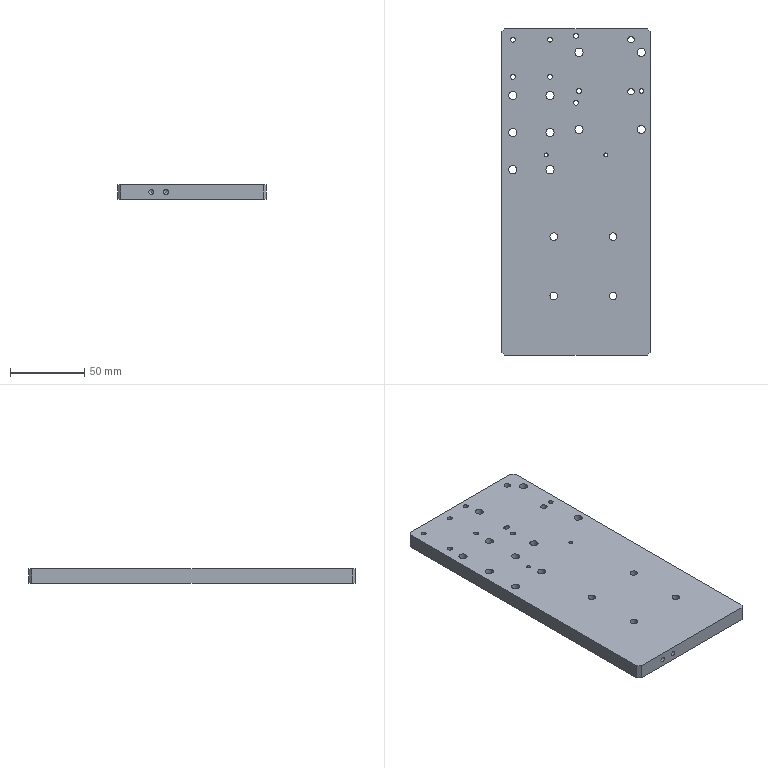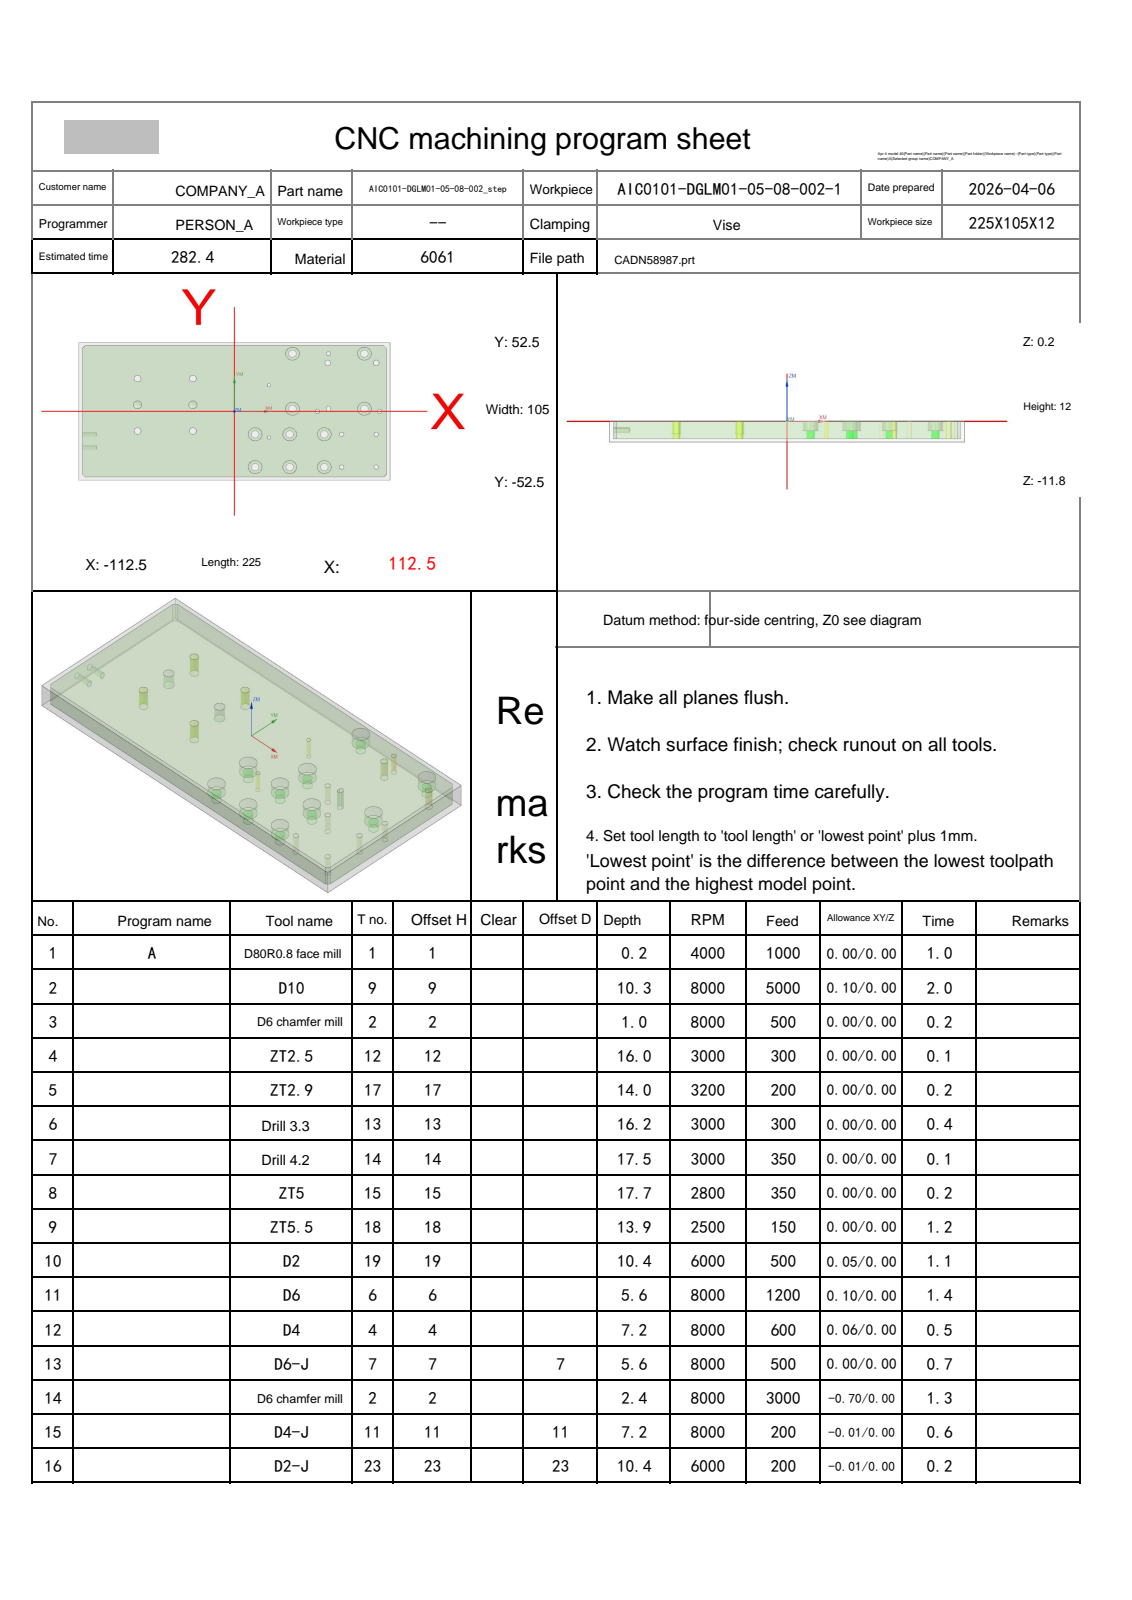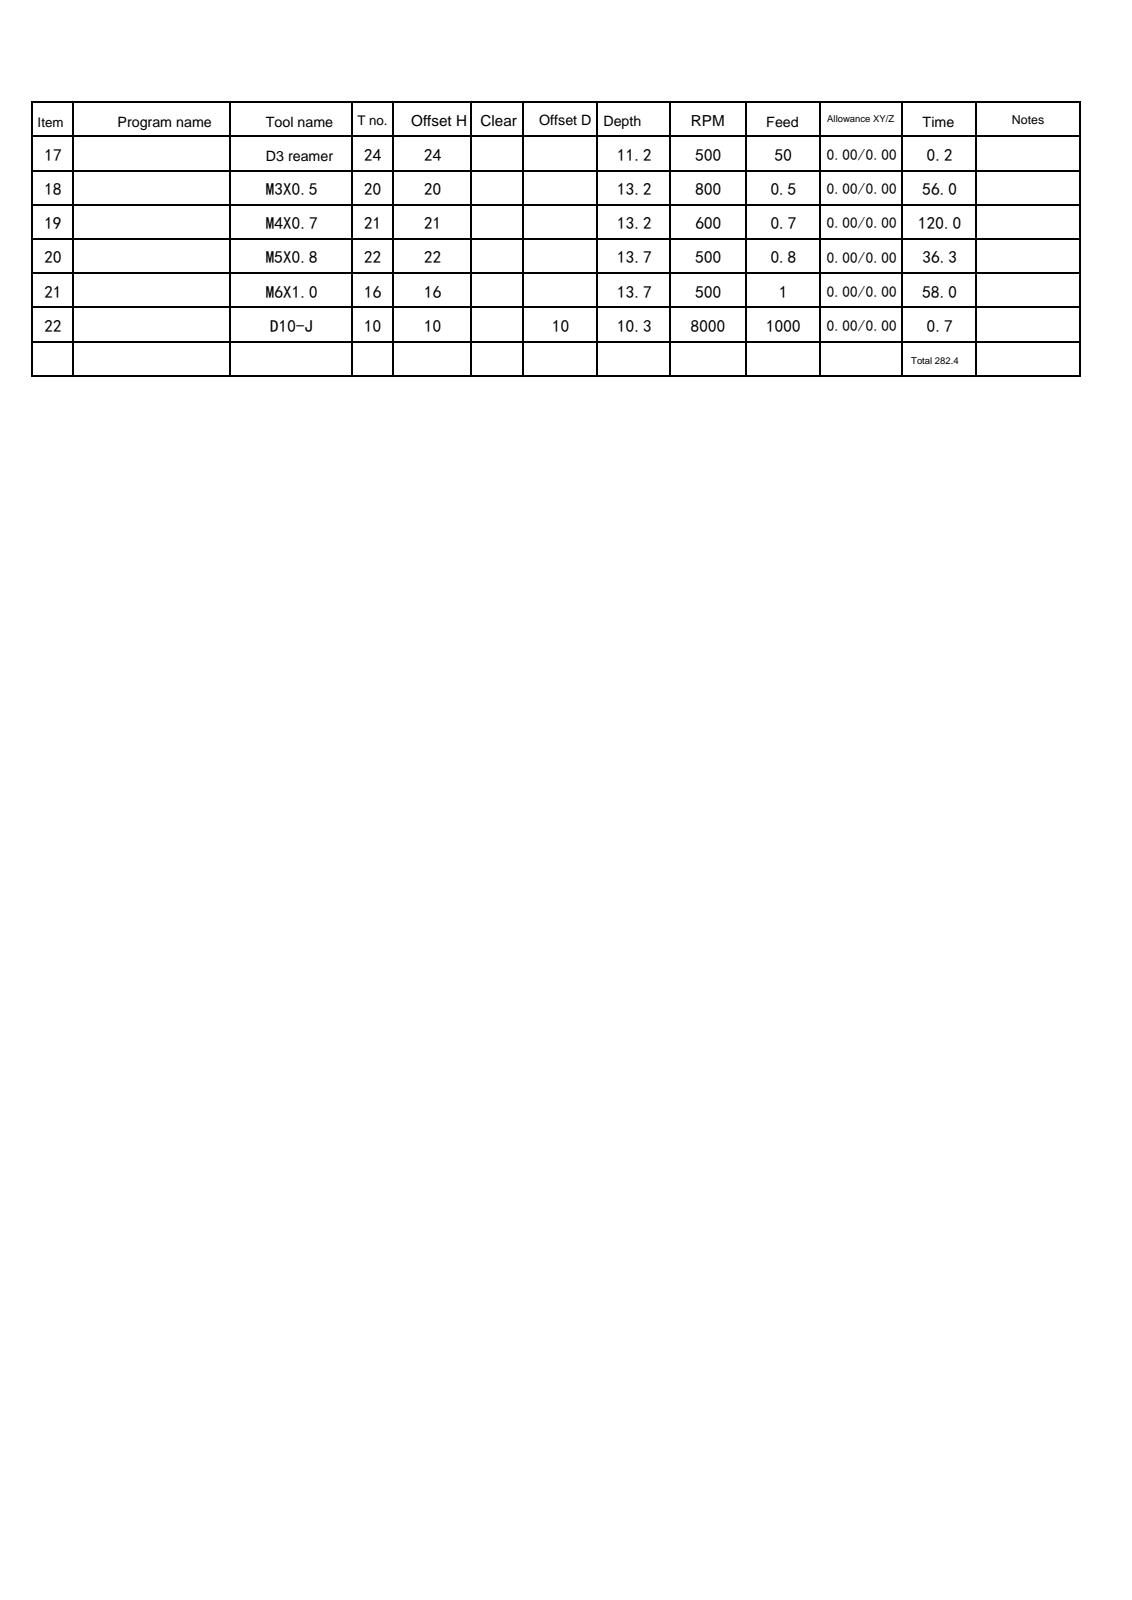NC program | NX | posted by the shop | part box 100 x 220 x 10 mm
Lines 1 to 1658 of 2500, first 1187 of 1656 lines:
%
O0001
(Machine time: 537.90 MIN)
(===Total Tool:21===)
(T1=D80R0.8 face mill D=80.  R=0.8  D-  H01 Z=-0.   )
(T9=D10     D=10.  R=0.   D-  H09 Z=-10.1 )
(T2=D6 chamfer mill   D=6.   R=0.   D-  H02 Z=-2.2  )
(T12=ZT2.5  D=2.5  DR_a=118 D-  H12 Z=-15.75)
(T17=ZT2.9  D=2.9  DR_a=120 D-  H17 Z=-13.84)
(T13=3.3 drill  D=3.3  DR_a=118 D-  H13 Z=-15.99)
(T14=4.2 drill  D=4.2  DR_a=118 D-  H14 Z=-17.26)
(T15=ZT5    D=5.   DR_a=118 D-  H15 Z=-17.5 )
(T18=ZT5.5  D=5.5  DR_a=118 D-  H18 Z=-13.65)
(T19=D2     D=2.   R=0.   D-  H19 Z=-10.2 )
(T6=D6      D=6.   R=0.   D-  H06 Z=-5.4  )
(T4=D4      D=4.   R=0.   D-  H04 Z=-7.   )
(T7=D6-J    D=6.   R=0.   D7  H07 Z=-5.4  )
(T11=D4-J   D=4.   R=0.   D11 H11 Z=-7.   )
(T23=D2-J   D=2.   R=0.   D23 H23 Z=-10.2 )
(T24=D3 reamer   D=3.   DR_a=180 D-  H24 Z=-11.  )
(T20=M3X0.5 D=2.5  DR_a=180 D-  H20 Z=-13.  )
(T21=M4X0.7 D=3.3  DR_a=180 D-  H21 Z=-13.  )
(T22=M5X0.8 D=4.2  DR_a=180 D-  H22 Z=-13.5 )
(T16=M6X1.0 D=5.   DR_a=180 D-  H16 Z=-13.5 )
(T10=D10-J  D=10.  R=0.   D10 H10 Z=-10.1 )
G80 G90 G17 G49 G40
G91 G28 Z0
M01
N1 T01 M06
(D80R0.8 face mill  D=80. R=0.8 H=01 ce=0.00 di=0.00)
G00 G90 G54 X-155. Y45. M03 S4000
G43 H01 Z20.
M08
Z2.
G01 Z0.0 F1000.
X-150.
X150.
Y0.0
X-150.
Y-45.
X150.
X155.
Z2.
G00 Z20.
G91 G28 Z0.0
M05
M09
G91 G28 Z0.0
M01
N2 T09 M06
(D10  D=10. R=0. H=09 ce=0.10 di=0.00)
G00 G90 G54 X0.0 Y55.1 M03 S8000
G43 H09 Z20.
M08
Z.5
G01 X108. Z.377 F5000.
G02 X111.606 Y53.606 Z.373 I0.0 J-5.1
G01 X113.606 Y51.606 Z.37
G02 X114.953 Y49.214 Z.367 I-3.606 J-3.606
X115.1 Y48. Z.365 I-4.953 J-1.214
G01 Y-48. Z.256
G02 X113.606 Y-51.606 Z.252 I-5.1 J0.0
G01 X111.606 Y-53.606 Z.249
G02 X108. Y-55.1 Z.244 I-3.606 J3.606
G01 X-108. Z-.001
G02 X-111.606 Y-53.606 Z-.006 I0.0 J5.1
G01 X-113.606 Y-51.606 Z-.009
G02 X-115.1 Y-48. Z-.013 I3.606 J3.606
G01 Y48. Z-.122
G02 X-113.606 Y51.606 Z-.127 I5.1 J0.0
G01 X-111.606 Y53.606 Z-.13
G02 X-108. Y55.1 Z-.135 I3.606 J-3.606
G01 X108. Z-.38
G02 X111.606 Y53.606 Z-.384 I0.0 J-5.1
G01 X113.606 Y51.606 Z-.387
G02 X114.953 Y49.214 Z-.391 I-3.606 J-3.606
X115.1 Y48. Z-.392 I-4.953 J-1.214
G01 Y-48. Z-.501
G02 X113.606 Y-51.606 Z-.505 I-5.1 J0.0
G01 X111.606 Y-53.606 Z-.509
G02 X108. Y-55.1 Z-.513 I-3.606 J3.606
G01 X-108. Z-.758
G02 X-111.606 Y-53.606 Z-.763 I0.0 J5.1
G01 X-113.606 Y-51.606 Z-.766
G02 X-115.1 Y-48. Z-.771 I3.606 J3.606
G01 Y48. Z-.879
G02 X-113.606 Y51.606 Z-.884 I5.1 J0.0
G01 X-111.606 Y53.606 Z-.887
G02 X-108. Y55.1 Z-.892 I3.606 J-3.606
G01 X108. Z-1.137
G02 X111.606 Y53.606 Z-1.141 I0.0 J-5.1
G01 X113.606 Y51.606 Z-1.145
G02 X114.953 Y49.214 Z-1.148 I-3.606 J-3.606
X115.1 Y48. Z-1.149 I-4.953 J-1.214
G01 Y-48. Z-1.258
G02 X113.606 Y-51.606 Z-1.263 I-5.1 J0.0
G01 X111.606 Y-53.606 Z-1.266
G02 X108. Y-55.1 Z-1.27 I-3.606 J3.606
G01 X-108. Z-1.515
G02 X-111.606 Y-53.606 Z-1.52 I0.0 J5.1
G01 X-113.606 Y-51.606 Z-1.523
G02 X-115.1 Y-48. Z-1.528 I3.606 J3.606
G01 Y48. Z-1.637
G02 X-113.606 Y51.606 Z-1.641 I5.1 J0.0
G01 X-111.606 Y53.606 Z-1.644
G02 X-108. Y55.1 Z-1.649 I3.606 J-3.606
G01 X108. Z-1.894
G02 X111.606 Y53.606 Z-1.899 I0.0 J-5.1
G01 X113.606 Y51.606 Z-1.902
G02 X114.953 Y49.214 Z-1.905 I-3.606 J-3.606
X115.1 Y48. Z-1.906 I-4.953 J-1.214
G01 Y-48. Z-2.015
G02 X113.606 Y-51.606 Z-2.02 I-5.1 J0.0
G01 X111.606 Y-53.606 Z-2.023
G02 X108. Y-55.1 Z-2.027 I-3.606 J3.606
G01 X-108. Z-2.273
G02 X-111.606 Y-53.606 Z-2.277 I0.0 J5.1
G01 X-113.606 Y-51.606 Z-2.28
G02 X-115.1 Y-48. Z-2.285 I3.606 J3.606
G01 Y48. Z-2.394
G02 X-113.606 Y51.606 Z-2.398 I5.1 J0.0
G01 X-111.606 Y53.606 Z-2.401
G02 X-108. Y55.1 Z-2.406 I3.606 J-3.606
G01 X108. Z-2.651
G02 X111.606 Y53.606 Z-2.656 I0.0 J-5.1
G01 X113.606 Y51.606 Z-2.659
G02 X114.953 Y49.214 Z-2.662 I-3.606 J-3.606
X115.1 Y48. Z-2.663 I-4.953 J-1.214
G01 Y-48. Z-2.772
G02 X113.606 Y-51.606 Z-2.777 I-5.1 J0.0
G01 X111.606 Y-53.606 Z-2.78
G02 X108. Y-55.1 Z-2.785 I-3.606 J3.606
G01 X-108. Z-3.03
G02 X-111.606 Y-53.606 Z-3.034 I0.0 J5.1
G01 X-113.606 Y-51.606 Z-3.037
G02 X-115.1 Y-48. Z-3.042 I3.606 J3.606
G01 Y48. Z-3.151
G02 X-113.606 Y51.606 Z-3.155 I5.1 J0.0
G01 X-111.606 Y53.606 Z-3.159
G02 X-108. Y55.1 Z-3.163 I3.606 J-3.606
G01 X108. Z-3.408
G02 X111.606 Y53.606 Z-3.413 I0.0 J-5.1
G01 X113.606 Y51.606 Z-3.416
G02 X114.953 Y49.214 Z-3.419 I-3.606 J-3.606
X115.1 Y48. Z-3.421 I-4.953 J-1.214
G01 Y-48. Z-3.529
G02 X113.606 Y-51.606 Z-3.534 I-5.1 J0.0
G01 X111.606 Y-53.606 Z-3.537
G02 X108. Y-55.1 Z-3.542 I-3.606 J3.606
G01 X-108. Z-3.787
G02 X-111.606 Y-53.606 Z-3.791 I0.0 J5.1
G01 X-113.606 Y-51.606 Z-3.795
G02 X-115.1 Y-48. Z-3.799 I3.606 J3.606
G01 Y48. Z-3.908
G02 X-113.606 Y51.606 Z-3.913 I5.1 J0.0
G01 X-111.606 Y53.606 Z-3.916
G02 X-108. Y55.1 Z-3.92 I3.606 J-3.606
G01 X108. Z-4.165
G02 X111.606 Y53.606 Z-4.17 I0.0 J-5.1
G01 X113.606 Y51.606 Z-4.173
G02 X114.953 Y49.214 Z-4.176 I-3.606 J-3.606
X115.1 Y48. Z-4.178 I-4.953 J-1.214
G01 Y-48. Z-4.287
G02 X113.606 Y-51.606 Z-4.291 I-5.1 J0.0
G01 X111.606 Y-53.606 Z-4.294
G02 X108. Y-55.1 Z-4.299 I-3.606 J3.606
G01 X-108. Z-4.544
G02 X-111.606 Y-53.606 Z-4.549 I0.0 J5.1
G01 X-113.606 Y-51.606 Z-4.552
G02 X-115.1 Y-48. Z-4.556 I3.606 J3.606
G01 Y48. Z-4.665
G02 X-113.606 Y51.606 Z-4.67 I5.1 J0.0
G01 X-111.606 Y53.606 Z-4.673
G02 X-108. Y55.1 Z-4.677 I3.606 J-3.606
G01 X108. Z-4.923
G02 X111.606 Y53.606 Z-4.927 I0.0 J-5.1
G01 X113.606 Y51.606 Z-4.93
G02 X114.953 Y49.214 Z-4.933 I-3.606 J-3.606
X115.1 Y48. Z-4.935 I-4.953 J-1.214
G01 Y-48. Z-5.044
G02 X113.606 Y-51.606 Z-5.048 I-5.1 J0.0
G01 X111.606 Y-53.606 Z-5.051
G02 X108. Y-55.1 Z-5.056 I-3.606 J3.606
G01 X-108. Z-5.301
G02 X-111.606 Y-53.606 Z-5.306 I0.0 J5.1
G01 X-113.606 Y-51.606 Z-5.309
G02 X-115.1 Y-48. Z-5.313 I3.606 J3.606
G01 Y48. Z-5.422
G02 X-113.606 Y51.606 Z-5.427 I5.1 J0.0
G01 X-111.606 Y53.606 Z-5.43
G02 X-108. Y55.1 Z-5.435 I3.606 J-3.606
G01 X108. Z-5.68
G02 X111.606 Y53.606 Z-5.684 I0.0 J-5.1
G01 X113.606 Y51.606 Z-5.687
G02 X114.953 Y49.214 Z-5.691 I-3.606 J-3.606
X115.1 Y48. Z-5.692 I-4.953 J-1.214
G01 Y-48. Z-5.801
G02 X113.606 Y-51.606 Z-5.805 I-5.1 J0.0
G01 X111.606 Y-53.606 Z-5.809
G02 X108. Y-55.1 Z-5.813 I-3.606 J3.606
G01 X-108. Z-6.058
G02 X-111.606 Y-53.606 Z-6.063 I0.0 J5.1
G01 X-113.606 Y-51.606 Z-6.066
G02 X-115.1 Y-48. Z-6.071 I3.606 J3.606
G01 Y48. Z-6.179
G02 X-113.606 Y51.606 Z-6.184 I5.1 J0.0
G01 X-111.606 Y53.606 Z-6.187
G02 X-108. Y55.1 Z-6.192 I3.606 J-3.606
G01 X108. Z-6.437
G02 X111.606 Y53.606 Z-6.441 I0.0 J-5.1
G01 X113.606 Y51.606 Z-6.445
G02 X114.953 Y49.214 Z-6.448 I-3.606 J-3.606
X115.1 Y48. Z-6.449 I-4.953 J-1.214
G01 Y-48. Z-6.558
G02 X113.606 Y-51.606 Z-6.563 I-5.1 J0.0
G01 X111.606 Y-53.606 Z-6.566
G02 X108. Y-55.1 Z-6.57 I-3.606 J3.606
G01 X-108. Z-6.815
G02 X-111.606 Y-53.606 Z-6.82 I0.0 J5.1
G01 X-113.606 Y-51.606 Z-6.823
G02 X-115.1 Y-48. Z-6.828 I3.606 J3.606
G01 Y48. Z-6.937
G02 X-113.606 Y51.606 Z-6.941 I5.1 J0.0
G01 X-111.606 Y53.606 Z-6.944
G02 X-108. Y55.1 Z-6.949 I3.606 J-3.606
G01 X108. Z-7.194
G02 X111.606 Y53.606 Z-7.199 I0.0 J-5.1
G01 X113.606 Y51.606 Z-7.202
G02 X114.953 Y49.214 Z-7.205 I-3.606 J-3.606
X115.1 Y48. Z-7.206 I-4.953 J-1.214
G01 Y-48. Z-7.315
G02 X113.606 Y-51.606 Z-7.32 I-5.1 J0.0
G01 X111.606 Y-53.606 Z-7.323
G02 X108. Y-55.1 Z-7.327 I-3.606 J3.606
G01 X-108. Z-7.573
G02 X-111.606 Y-53.606 Z-7.577 I0.0 J5.1
G01 X-113.606 Y-51.606 Z-7.58
G02 X-115.1 Y-48. Z-7.585 I3.606 J3.606
G01 Y48. Z-7.694
G02 X-113.606 Y51.606 Z-7.698 I5.1 J0.0
G01 X-111.606 Y53.606 Z-7.701
G02 X-108. Y55.1 Z-7.706 I3.606 J-3.606
G01 X108. Z-7.951
G02 X111.606 Y53.606 Z-7.956 I0.0 J-5.1
G01 X113.606 Y51.606 Z-7.959
G02 X114.953 Y49.214 Z-7.962 I-3.606 J-3.606
X115.1 Y48. Z-7.963 I-4.953 J-1.214
G01 Y-48. Z-8.072
G02 X113.606 Y-51.606 Z-8.077 I-5.1 J0.0
G01 X111.606 Y-53.606 Z-8.08
G02 X108. Y-55.1 Z-8.085 I-3.606 J3.606
G01 X-108. Z-8.33
G02 X-111.606 Y-53.606 Z-8.334 I0.0 J5.1
G01 X-113.606 Y-51.606 Z-8.337
G02 X-115.1 Y-48. Z-8.342 I3.606 J3.606
G01 Y48. Z-8.451
G02 X-113.606 Y51.606 Z-8.455 I5.1 J0.0
G01 X-111.606 Y53.606 Z-8.459
G02 X-108. Y55.1 Z-8.463 I3.606 J-3.606
G01 X108. Z-8.708
G02 X111.606 Y53.606 Z-8.713 I0.0 J-5.1
G01 X113.606 Y51.606 Z-8.716
G02 X114.953 Y49.214 Z-8.719 I-3.606 J-3.606
X115.1 Y48. Z-8.721 I-4.953 J-1.214
G01 Y-48. Z-8.829
G02 X113.606 Y-51.606 Z-8.834 I-5.1 J0.0
G01 X111.606 Y-53.606 Z-8.837
G02 X108. Y-55.1 Z-8.842 I-3.606 J3.606
G01 X-108. Z-9.087
G02 X-111.606 Y-53.606 Z-9.091 I0.0 J5.1
G01 X-113.606 Y-51.606 Z-9.095
G02 X-115.1 Y-48. Z-9.099 I3.606 J3.606
G01 Y48. Z-9.208
G02 X-113.606 Y51.606 Z-9.213 I5.1 J0.0
G01 X-111.606 Y53.606 Z-9.216
G02 X-108. Y55.1 Z-9.22 I3.606 J-3.606
G01 X108. Z-9.465
G02 X111.606 Y53.606 Z-9.47 I0.0 J-5.1
G01 X113.606 Y51.606 Z-9.473
G02 X114.953 Y49.214 Z-9.476 I-3.606 J-3.606
X115.1 Y48. Z-9.478 I-4.953 J-1.214
G01 Y-48. Z-9.587
G02 X113.606 Y-51.606 Z-9.591 I-5.1 J0.0
G01 X111.606 Y-53.606 Z-9.594
G02 X108. Y-55.1 Z-9.599 I-3.606 J3.606
G01 X-108. Z-9.844
G02 X-111.606 Y-53.606 Z-9.849 I0.0 J5.1
G01 X-113.606 Y-51.606 Z-9.852
G02 X-115.1 Y-48. Z-9.856 I3.606 J3.606
G01 Y48. Z-9.965
G02 X-113.606 Y51.606 Z-9.97 I5.1 J0.0
G01 X-111.606 Y53.606 Z-9.973
G02 X-108. Y55.1 Z-9.977 I3.606 J-3.606
G01 X0.0 Z-10.1
X108.
G02 X111.606 Y53.606 I0.0 J-5.1
G01 X113.606 Y51.606
G02 X115.1 Y48. I-3.606 J-3.606
G01 Y-48.
G02 X113.606 Y-51.606 I-5.1 J0.0
G01 X111.606 Y-53.606
G02 X108. Y-55.1 I-3.606 J3.606
G01 X-108.
G02 X-111.606 Y-53.606 I0.0 J5.1
G01 X-113.606 Y-51.606
G02 X-115.1 Y-48. I3.606 J3.606
G01 Y48.
G02 X-113.606 Y51.606 I5.1 J0.0
G01 X-111.606 Y53.606
G02 X-108. Y55.1 I3.606 J-3.606
G01 X0.0
X.5
Z-9.1
G00 Z20.
G91 G28 Z0.0
M05
M09
G91 G28 Z0.0
M01
N3 T02 M06
(D6 chamfer mill  D=6. R=0. H=02 ce=0.00 di=0.00)
G00 G90 G54 X102.5 Y37. M03 S8000
G43 H02 Z20.
M08
G98 G81 X102.5 Y37. Z-.8 R1. F500.
X94. Y44.
X68.
X67.5 Y37.
X42. Y44.
X25. Y20.
X42. Y2.
X60. Y0.0
X65. Y-17.5
X77.5
X94. Y2.
X105. Y0.0
X102.5 Y-17.5
Y-42.5
X77.5
X65.
X40.
Y-17.5
X25. Y-20.
X15. Y-17.5
Y-42.5
X-30. Y-15.
Y5.
Y25.
X-70.
Y5.
Y-15.
X68. Y2.5
G80
G00 Z20.
G91 G28 Z0.0
M05
M09
G91 G28 Z0.0
M01
N4 T12 M06
(ZT2.5 D=2.5 DR_a=118 H=12)
G00 G90 G54 X25. Y-20. M03 S3000
G43 H12 Z20.
M08
G98 G83 X25. Y-20. Z-15.751 R1. F300. Q2.
Y20.
G80
G00 Z20.
G91 G28 Z0.0
M05
M09
G91 G28 Z0.0
M01
N5 T17 M06
(ZT2.9 D=2.9 DR_a=120 H=17)
G00 G90 G54 X68. Y44. M03 S3200
G43 H17 Z20.
M08
G98 G83 X68. Y44. Z-13.837 R1. F200. Q2.
Y2.5
G80
G00 Z20.
G91 G28 Z0.0
M05
M09
G91 G28 Z0.0
M01
N6 T13 M06
(3.3 drill D=3.3 DR_a=118 H=13)
G00 G90 G54 X60. Y0.0 M03 S3000
G43 H13 Z20.
M08
G98 G83 X60. Y0.0 Z-15.991 R1. F300. Q2.
X77.5 Y-17.5
Y-42.5
X102.5
Y-17.5
X105. Y0.0
G80
G00 Z20.
G91 G28 Z0.0
M05
M09
G91 G28 Z0.0
M01
N7 T14 M06
(4.2 drill D=4.2 DR_a=118 H=14)
G00 G90 G54 X67.5 Y37. M03 S3000
G43 H14 Z20.
M08
G98 G83 X67.5 Y37. Z-17.262 R1. F350. Q3.
X102.5
G80
G00 Z20.
G91 G28 Z0.0
M05
M09
G91 G28 Z0.0
M01
N8 T15 M06
(ZT5 D=5. DR_a=118 H=15)
G00 G90 G54 X-30. Y25. M03 S2800
G43 H15 Z20.
M08
G98 G83 X-30. Y25. Z-17.502 R1. F350. Q3.
X-70.
Y-15.
X-30.
G80
G00 Z20.
G91 G28 Z0.0
M05
M09
G91 G28 Z0.0
M01
N9 T18 M06
(ZT5.5 D=5.5 DR_a=118 H=18)
G00 G90 G54 X42. Y44. M03 S1200
G43 H18 Z20.
M08
G98 G83 X42. Y44. Z-13.652 R1. F150. Q2.
Y2.
X40. Y-17.5
X15.
Y-42.5
X40.
X65.
Y-17.5
X94. Y2.
Y44.
G80
G00 Z20.
G00 G90 X-30. Y5. M03 S2500
Z20.
G98 G83 X-30. Y5. Z-8.703 R1. F150. Q2.
X-70.
G80
G00 Z20.
G91 G28 Z0.0
M05
M09
G91 G28 Z0.0
M01
N10 T19 M06
(D2  D=2. R=0. H=19 ce=0.05 di=0.00)
G00 G90 G54 X68.45 Y2. M03 S6000
G43 H19 Z20.
M08
Z.5
G01 Y2.5 Z.49 F500.
G03 X68. Y2.95 Z.475 I-.45 J0.0
X67.55 Y2.5 Z.46 I0.0 J-.45
G01 Y1.5 Z.44
G03 X68. Y1.05 Z.425 I.45 J0.0
X68.45 Y1.5 Z.41 I0.0 J.45
G01 Y2.5 Z.39
G03 X68. Y2.95 Z.375 I-.45 J0.0
X67.55 Y2.5 Z.36 I0.0 J-.45
G01 Y1.5 Z.34
G03 X68. Y1.05 Z.325 I.45 J0.0
X68.45 Y1.5 Z.31 I0.0 J.45
G01 Y2.5 Z.29
G03 X68. Y2.95 Z.275 I-.45 J0.0
X67.55 Y2.5 Z.26 I0.0 J-.45
G01 Y1.5 Z.24
G03 X68. Y1.05 Z.225 I.45 J0.0
X68.45 Y1.5 Z.21 I0.0 J.45
G01 Y2.5 Z.19
G03 X68. Y2.95 Z.175 I-.45 J0.0
X67.55 Y2.5 Z.16 I0.0 J-.45
G01 Y1.5 Z.14
G03 X68. Y1.05 Z.125 I.45 J0.0
X68.45 Y1.5 Z.11 I0.0 J.45
G01 Y2.5 Z.09
G03 X68. Y2.95 Z.075 I-.45 J0.0
X67.55 Y2.5 Z.06 I0.0 J-.45
G01 Y1.5 Z.04
G03 X68. Y1.05 Z.025 I.45 J0.0
X68.45 Y1.5 Z.01 I0.0 J.45
G01 Y2.5 Z-.01
G03 X68. Y2.95 Z-.025 I-.45 J0.0
X67.55 Y2.5 Z-.04 I0.0 J-.45
G01 Y1.5 Z-.06
G03 X68. Y1.05 Z-.075 I.45 J0.0
X68.45 Y1.5 Z-.09 I0.0 J.45
G01 Y2.5 Z-.11
G03 X68. Y2.95 Z-.125 I-.45 J0.0
X67.55 Y2.5 Z-.14 I0.0 J-.45
G01 Y1.5 Z-.16
G03 X68. Y1.05 Z-.175 I.45 J0.0
X68.45 Y1.5 Z-.19 I0.0 J.45
G01 Y2.5 Z-.21
G03 X68. Y2.95 Z-.225 I-.45 J0.0
X67.55 Y2.5 Z-.24 I0.0 J-.45
G01 Y1.5 Z-.26
G03 X68. Y1.05 Z-.275 I.45 J0.0
X68.45 Y1.5 Z-.29 I0.0 J.45
G01 Y2.5 Z-.31
G03 X68. Y2.95 Z-.325 I-.45 J0.0
X67.55 Y2.5 Z-.34 I0.0 J-.45
G01 Y1.5 Z-.36
G03 X68. Y1.05 Z-.375 I.45 J0.0
X68.45 Y1.5 Z-.39 I0.0 J.45
G01 Y2.5 Z-.41
G03 X68. Y2.95 Z-.425 I-.45 J0.0
X67.55 Y2.5 Z-.44 I0.0 J-.45
G01 Y1.5 Z-.46
G03 X68. Y1.05 Z-.475 I.45 J0.0
X68.45 Y1.5 Z-.49 I0.0 J.45
G01 Y2.5 Z-.51
G03 X68. Y2.95 Z-.525 I-.45 J0.0
X67.55 Y2.5 Z-.54 I0.0 J-.45
G01 Y1.5 Z-.56
G03 X68. Y1.05 Z-.575 I.45 J0.0
X68.45 Y1.5 Z-.59 I0.0 J.45
G01 Y2.5 Z-.61
G03 X68. Y2.95 Z-.625 I-.45 J0.0
X67.55 Y2.5 Z-.64 I0.0 J-.45
G01 Y1.5 Z-.66
G03 X68. Y1.05 Z-.675 I.45 J0.0
X68.45 Y1.5 Z-.69 I0.0 J.45
G01 Y2.5 Z-.71
G03 X68. Y2.95 Z-.725 I-.45 J0.0
X67.55 Y2.5 Z-.74 I0.0 J-.45
G01 Y1.5 Z-.76
G03 X68. Y1.05 Z-.775 I.45 J0.0
X68.45 Y1.5 Z-.79 I0.0 J.45
G01 Y2.5 Z-.81
G03 X68. Y2.95 Z-.825 I-.45 J0.0
X67.55 Y2.5 Z-.84 I0.0 J-.45
G01 Y1.5 Z-.86
G03 X68. Y1.05 Z-.875 I.45 J0.0
X68.45 Y1.5 Z-.89 I0.0 J.45
G01 Y2.5 Z-.91
G03 X68. Y2.95 Z-.925 I-.45 J0.0
X67.55 Y2.5 Z-.94 I0.0 J-.45
G01 Y1.5 Z-.96
G03 X68. Y1.05 Z-.975 I.45 J0.0
X68.45 Y1.5 Z-.99 I0.0 J.45
G01 Y2.5 Z-1.01
G03 X68. Y2.95 Z-1.025 I-.45 J0.0
X67.55 Y2.5 Z-1.04 I0.0 J-.45
G01 Y1.5 Z-1.06
G03 X68. Y1.05 Z-1.075 I.45 J0.0
X68.45 Y1.5 Z-1.09 I0.0 J.45
G01 Y2.5 Z-1.11
G03 X68. Y2.95 Z-1.125 I-.45 J0.0
X67.55 Y2.5 Z-1.14 I0.0 J-.45
G01 Y1.5 Z-1.16
G03 X68. Y1.05 Z-1.175 I.45 J0.0
X68.45 Y1.5 Z-1.19 I0.0 J.45
G01 Y2.5 Z-1.21
G03 X68. Y2.95 Z-1.225 I-.45 J0.0
X67.55 Y2.5 Z-1.24 I0.0 J-.45
G01 Y1.5 Z-1.26
G03 X68. Y1.05 Z-1.275 I.45 J0.0
X68.45 Y1.5 Z-1.29 I0.0 J.45
G01 Y2.5 Z-1.31
G03 X68. Y2.95 Z-1.325 I-.45 J0.0
X67.55 Y2.5 Z-1.34 I0.0 J-.45
G01 Y1.5 Z-1.36
G03 X68. Y1.05 Z-1.375 I.45 J0.0
X68.45 Y1.5 Z-1.39 I0.0 J.45
G01 Y2.5 Z-1.41
G03 X68. Y2.95 Z-1.425 I-.45 J0.0
X67.55 Y2.5 Z-1.44 I0.0 J-.45
G01 Y1.5 Z-1.46
G03 X68. Y1.05 Z-1.475 I.45 J0.0
X68.45 Y1.5 Z-1.49 I0.0 J.45
G01 Y2.5 Z-1.51
G03 X68. Y2.95 Z-1.525 I-.45 J0.0
X67.55 Y2.5 Z-1.54 I0.0 J-.45
G01 Y1.5 Z-1.56
G03 X68. Y1.05 Z-1.575 I.45 J0.0
X68.45 Y1.5 Z-1.59 I0.0 J.45
G01 Y2.5 Z-1.61
G03 X68. Y2.95 Z-1.625 I-.45 J0.0
X67.55 Y2.5 Z-1.64 I0.0 J-.45
G01 Y1.5 Z-1.66
G03 X68. Y1.05 Z-1.675 I.45 J0.0
X68.45 Y1.5 Z-1.69 I0.0 J.45
G01 Y2.5 Z-1.71
G03 X68. Y2.95 Z-1.725 I-.45 J0.0
X67.55 Y2.5 Z-1.74 I0.0 J-.45
G01 Y1.5 Z-1.76
G03 X68. Y1.05 Z-1.775 I.45 J0.0
X68.45 Y1.5 Z-1.79 I0.0 J.45
G01 Y2.5 Z-1.81
G03 X68. Y2.95 Z-1.825 I-.45 J0.0
X67.55 Y2.5 Z-1.84 I0.0 J-.45
G01 Y1.5 Z-1.86
G03 X68. Y1.05 Z-1.875 I.45 J0.0
X68.45 Y1.5 Z-1.89 I0.0 J.45
G01 Y2.5 Z-1.91
G03 X68. Y2.95 Z-1.925 I-.45 J0.0
X67.55 Y2.5 Z-1.94 I0.0 J-.45
G01 Y1.5 Z-1.96
G03 X68. Y1.05 Z-1.975 I.45 J0.0
X68.45 Y1.5 Z-1.99 I0.0 J.45
G01 Y2.5 Z-2.01
G03 X68. Y2.95 Z-2.025 I-.45 J0.0
X67.55 Y2.5 Z-2.04 I0.0 J-.45
G01 Y1.5 Z-2.06
G03 X68. Y1.05 Z-2.075 I.45 J0.0
X68.45 Y1.5 Z-2.09 I0.0 J.45
G01 Y2.5 Z-2.11
G03 X68. Y2.95 Z-2.125 I-.45 J0.0
X67.55 Y2.5 Z-2.14 I0.0 J-.45
G01 Y1.5 Z-2.16
G03 X68. Y1.05 Z-2.175 I.45 J0.0
X68.45 Y1.5 Z-2.19 I0.0 J.45
G01 Y2.5 Z-2.21
G03 X68. Y2.95 Z-2.225 I-.45 J0.0
X67.55 Y2.5 Z-2.24 I0.0 J-.45
G01 Y1.5 Z-2.26
G03 X68. Y1.05 Z-2.275 I.45 J0.0
X68.45 Y1.5 Z-2.29 I0.0 J.45
G01 Y2.5 Z-2.31
G03 X68. Y2.95 Z-2.325 I-.45 J0.0
X67.55 Y2.5 Z-2.34 I0.0 J-.45
G01 Y1.5 Z-2.36
G03 X68. Y1.05 Z-2.375 I.45 J0.0
X68.45 Y1.5 Z-2.39 I0.0 J.45
G01 Y2.5 Z-2.41
G03 X68. Y2.95 Z-2.425 I-.45 J0.0
X67.55 Y2.5 Z-2.44 I0.0 J-.45
G01 Y1.5 Z-2.46
G03 X68. Y1.05 Z-2.475 I.45 J0.0
X68.45 Y1.5 Z-2.49 I0.0 J.45
G01 Y2.5 Z-2.51
G03 X68. Y2.95 Z-2.525 I-.45 J0.0
X67.55 Y2.5 Z-2.54 I0.0 J-.45
G01 Y1.5 Z-2.56
G03 X68. Y1.05 Z-2.575 I.45 J0.0
X68.45 Y1.5 Z-2.59 I0.0 J.45
G01 Y2.5 Z-2.61
G03 X68. Y2.95 Z-2.625 I-.45 J0.0
X67.55 Y2.5 Z-2.64 I0.0 J-.45
G01 Y1.5 Z-2.66
G03 X68. Y1.05 Z-2.675 I.45 J0.0
X68.45 Y1.5 Z-2.69 I0.0 J.45
G01 Y2.5 Z-2.71
G03 X68. Y2.95 Z-2.725 I-.45 J0.0
X67.55 Y2.5 Z-2.74 I0.0 J-.45
G01 Y1.5 Z-2.76
G03 X68. Y1.05 Z-2.775 I.45 J0.0
X68.45 Y1.5 Z-2.79 I0.0 J.45
G01 Y2.5 Z-2.81
G03 X68. Y2.95 Z-2.825 I-.45 J0.0
X67.55 Y2.5 Z-2.84 I0.0 J-.45
G01 Y1.5 Z-2.86
G03 X68. Y1.05 Z-2.875 I.45 J0.0
X68.45 Y1.5 Z-2.89 I0.0 J.45
G01 Y2.5 Z-2.91
G03 X68. Y2.95 Z-2.925 I-.45 J0.0
X67.55 Y2.5 Z-2.94 I0.0 J-.45
G01 Y1.5 Z-2.96
G03 X68. Y1.05 Z-2.975 I.45 J0.0
X68.45 Y1.5 Z-2.99 I0.0 J.45
G01 Y2.5 Z-3.01
G03 X68. Y2.95 Z-3.025 I-.45 J0.0
X67.55 Y2.5 Z-3.04 I0.0 J-.45
G01 Y1.5 Z-3.06
G03 X68. Y1.05 Z-3.075 I.45 J0.0
X68.45 Y1.5 Z-3.09 I0.0 J.45
G01 Y2.5 Z-3.11
G03 X68. Y2.95 Z-3.125 I-.45 J0.0
X67.55 Y2.5 Z-3.14 I0.0 J-.45
G01 Y1.5 Z-3.16
G03 X68. Y1.05 Z-3.175 I.45 J0.0
X68.45 Y1.5 Z-3.19 I0.0 J.45
G01 Y2.5 Z-3.21
G03 X68. Y2.95 Z-3.225 I-.45 J0.0
X67.55 Y2.5 Z-3.24 I0.0 J-.45
G01 Y1.5 Z-3.26
G03 X68. Y1.05 Z-3.275 I.45 J0.0
X68.45 Y1.5 Z-3.29 I0.0 J.45
G01 Y2.5 Z-3.31
G03 X68. Y2.95 Z-3.325 I-.45 J0.0
X67.55 Y2.5 Z-3.34 I0.0 J-.45
G01 Y1.5 Z-3.36
G03 X68. Y1.05 Z-3.375 I.45 J0.0
X68.45 Y1.5 Z-3.39 I0.0 J.45
G01 Y2.5 Z-3.41
G03 X68. Y2.95 Z-3.425 I-.45 J0.0
X67.55 Y2.5 Z-3.44 I0.0 J-.45
G01 Y1.5 Z-3.46
G03 X68. Y1.05 Z-3.475 I.45 J0.0
X68.45 Y1.5 Z-3.49 I0.0 J.45
G01 Y2.5 Z-3.51
G03 X68. Y2.95 Z-3.525 I-.45 J0.0
X67.55 Y2.5 Z-3.54 I0.0 J-.45
G01 Y1.5 Z-3.56
G03 X68. Y1.05 Z-3.575 I.45 J0.0
X68.45 Y1.5 Z-3.59 I0.0 J.45
G01 Y2.5 Z-3.61
G03 X68. Y2.95 Z-3.625 I-.45 J0.0
X67.55 Y2.5 Z-3.64 I0.0 J-.45
G01 Y1.5 Z-3.66
G03 X68. Y1.05 Z-3.675 I.45 J0.0
X68.45 Y1.5 Z-3.69 I0.0 J.45
G01 Y2.5 Z-3.71
G03 X68. Y2.95 Z-3.725 I-.45 J0.0
X67.55 Y2.5 Z-3.74 I0.0 J-.45
G01 Y1.5 Z-3.76
G03 X68. Y1.05 Z-3.775 I.45 J0.0
X68.45 Y1.5 Z-3.79 I0.0 J.45
G01 Y2.5 Z-3.81
G03 X68. Y2.95 Z-3.825 I-.45 J0.0
X67.55 Y2.5 Z-3.84 I0.0 J-.45
G01 Y1.5 Z-3.86
G03 X68. Y1.05 Z-3.875 I.45 J0.0
X68.45 Y1.5 Z-3.89 I0.0 J.45
G01 Y2.5 Z-3.91
G03 X68. Y2.95 Z-3.925 I-.45 J0.0
X67.55 Y2.5 Z-3.94 I0.0 J-.45
G01 Y1.5 Z-3.96
G03 X68. Y1.05 Z-3.975 I.45 J0.0
X68.45 Y1.5 Z-3.99 I0.0 J.45
G01 Y2.5 Z-4.01
G03 X68. Y2.95 Z-4.025 I-.45 J0.0
X67.55 Y2.5 Z-4.04 I0.0 J-.45
G01 Y1.5 Z-4.06
G03 X68. Y1.05 Z-4.075 I.45 J0.0
X68.45 Y1.5 Z-4.09 I0.0 J.45
G01 Y2.5 Z-4.11
G03 X68. Y2.95 Z-4.125 I-.45 J0.0
X67.55 Y2.5 Z-4.14 I0.0 J-.45
G01 Y1.5 Z-4.16
G03 X68. Y1.05 Z-4.175 I.45 J0.0
X68.45 Y1.5 Z-4.19 I0.0 J.45
G01 Y2.5 Z-4.21
G03 X68. Y2.95 Z-4.225 I-.45 J0.0
X67.55 Y2.5 Z-4.24 I0.0 J-.45
G01 Y1.5 Z-4.26
G03 X68. Y1.05 Z-4.275 I.45 J0.0
X68.45 Y1.5 Z-4.29 I0.0 J.45
G01 Y2.5 Z-4.31
G03 X68. Y2.95 Z-4.325 I-.45 J0.0
X67.55 Y2.5 Z-4.34 I0.0 J-.45
G01 Y1.5 Z-4.36
G03 X68. Y1.05 Z-4.375 I.45 J0.0
X68.45 Y1.5 Z-4.39 I0.0 J.45
G01 Y2.5 Z-4.41
G03 X68. Y2.95 Z-4.425 I-.45 J0.0
X67.55 Y2.5 Z-4.44 I0.0 J-.45
G01 Y1.5 Z-4.46
G03 X68. Y1.05 Z-4.475 I.45 J0.0
X68.45 Y1.5 Z-4.49 I0.0 J.45
G01 Y2.5 Z-4.51
G03 X68. Y2.95 Z-4.525 I-.45 J0.0
X67.55 Y2.5 Z-4.54 I0.0 J-.45
G01 Y1.5 Z-4.56
G03 X68. Y1.05 Z-4.575 I.45 J0.0
X68.45 Y1.5 Z-4.59 I0.0 J.45
G01 Y2.5 Z-4.61
G03 X68. Y2.95 Z-4.625 I-.45 J0.0
X67.55 Y2.5 Z-4.64 I0.0 J-.45
G01 Y1.5 Z-4.66
G03 X68. Y1.05 Z-4.675 I.45 J0.0
X68.45 Y1.5 Z-4.69 I0.0 J.45
G01 Y2.5 Z-4.71
G03 X68. Y2.95 Z-4.725 I-.45 J0.0
X67.55 Y2.5 Z-4.74 I0.0 J-.45
G01 Y1.5 Z-4.76
G03 X68. Y1.05 Z-4.775 I.45 J0.0
X68.45 Y1.5 Z-4.79 I0.0 J.45
G01 Y2.5 Z-4.81
G03 X68. Y2.95 Z-4.825 I-.45 J0.0
X67.55 Y2.5 Z-4.84 I0.0 J-.45
G01 Y1.5 Z-4.86
G03 X68. Y1.05 Z-4.875 I.45 J0.0
X68.45 Y1.5 Z-4.89 I0.0 J.45
G01 Y2.5 Z-4.91
G03 X68. Y2.95 Z-4.925 I-.45 J0.0
X67.55 Y2.5 Z-4.94 I0.0 J-.45
G01 Y1.5 Z-4.96
G03 X68. Y1.05 Z-4.975 I.45 J0.0
X68.45 Y1.5 Z-4.99 I0.0 J.45
G01 Y2.5 Z-5.01
G03 X68. Y2.95 Z-5.025 I-.45 J0.0
X67.55 Y2.5 Z-5.04 I0.0 J-.45
G01 Y1.5 Z-5.06
G03 X68. Y1.05 Z-5.075 I.45 J0.0
X68.45 Y1.5 Z-5.09 I0.0 J.45
G01 Y2.5 Z-5.11
G03 X68. Y2.95 Z-5.125 I-.45 J0.0
X67.55 Y2.5 Z-5.14 I0.0 J-.45
G01 Y1.5 Z-5.16
G03 X68. Y1.05 Z-5.175 I.45 J0.0
X68.45 Y1.5 Z-5.19 I0.0 J.45
G01 Y2.5 Z-5.21
G03 X68. Y2.95 Z-5.225 I-.45 J0.0
X67.55 Y2.5 Z-5.24 I0.0 J-.45
G01 Y1.5 Z-5.26
G03 X68. Y1.05 Z-5.275 I.45 J0.0
X68.45 Y1.5 Z-5.29 I0.0 J.45
G01 Y2.5 Z-5.31
G03 X68. Y2.95 Z-5.325 I-.45 J0.0
X67.55 Y2.5 Z-5.34 I0.0 J-.45
G01 Y1.5 Z-5.36
G03 X68. Y1.05 Z-5.375 I.45 J0.0
X68.45 Y1.5 Z-5.39 I0.0 J.45
G01 Y2.5 Z-5.41
G03 X68. Y2.95 Z-5.425 I-.45 J0.0
X67.55 Y2.5 Z-5.44 I0.0 J-.45
G01 Y1.5 Z-5.46
G03 X68. Y1.05 Z-5.475 I.45 J0.0
X68.45 Y1.5 Z-5.49 I0.0 J.45
G01 Y2.5 Z-5.51
G03 X68. Y2.95 Z-5.525 I-.45 J0.0
X67.55 Y2.5 Z-5.54 I0.0 J-.45
G01 Y1.5 Z-5.56
G03 X68. Y1.05 Z-5.575 I.45 J0.0
X68.45 Y1.5 Z-5.59 I0.0 J.45
G01 Y2.5 Z-5.61
G03 X68. Y2.95 Z-5.625 I-.45 J0.0
X67.55 Y2.5 Z-5.64 I0.0 J-.45
G01 Y1.5 Z-5.66
G03 X68. Y1.05 Z-5.675 I.45 J0.0
X68.45 Y1.5 Z-5.69 I0.0 J.45
G01 Y2.5 Z-5.71
G03 X68. Y2.95 Z-5.725 I-.45 J0.0
X67.55 Y2.5 Z-5.74 I0.0 J-.45
G01 Y1.5 Z-5.76
G03 X68. Y1.05 Z-5.775 I.45 J0.0
X68.45 Y1.5 Z-5.79 I0.0 J.45
G01 Y2.5 Z-5.81
G03 X68. Y2.95 Z-5.825 I-.45 J0.0
X67.55 Y2.5 Z-5.84 I0.0 J-.45
G01 Y1.5 Z-5.86
G03 X68. Y1.05 Z-5.875 I.45 J0.0
X68.45 Y1.5 Z-5.89 I0.0 J.45
G01 Y2.5 Z-5.91
G03 X68. Y2.95 Z-5.925 I-.45 J0.0
X67.55 Y2.5 Z-5.94 I0.0 J-.45
G01 Y1.5 Z-5.96
G03 X68. Y1.05 Z-5.975 I.45 J0.0
X68.45 Y1.5 Z-5.99 I0.0 J.45
G01 Y2.5 Z-6.01
G03 X68. Y2.95 Z-6.025 I-.45 J0.0
X67.55 Y2.5 Z-6.04 I0.0 J-.45
G01 Y1.5 Z-6.06
G03 X68. Y1.05 Z-6.075 I.45 J0.0
X68.45 Y1.5 Z-6.09 I0.0 J.45
G01 Y2.5 Z-6.11
G03 X68. Y2.95 Z-6.125 I-.45 J0.0
X67.55 Y2.5 Z-6.14 I0.0 J-.45
G01 Y1.5 Z-6.16
G03 X68. Y1.05 Z-6.175 I.45 J0.0
X68.45 Y1.5 Z-6.19 I0.0 J.45
G01 Y2.5 Z-6.21
G03 X68. Y2.95 Z-6.225 I-.45 J0.0
X67.55 Y2.5 Z-6.24 I0.0 J-.45
G01 Y1.5 Z-6.26
G03 X68. Y1.05 Z-6.275 I.45 J0.0
X68.45 Y1.5 Z-6.29 I0.0 J.45
G01 Y2.5 Z-6.31
G03 X68. Y2.95 Z-6.325 I-.45 J0.0
X67.55 Y2.5 Z-6.34 I0.0 J-.45
G01 Y1.5 Z-6.36
G03 X68. Y1.05 Z-6.375 I.45 J0.0
X68.45 Y1.5 Z-6.39 I0.0 J.45
G01 Y2.5 Z-6.41
G03 X68. Y2.95 Z-6.425 I-.45 J0.0
X67.55 Y2.5 Z-6.44 I0.0 J-.45
G01 Y1.5 Z-6.46
G03 X68. Y1.05 Z-6.475 I.45 J0.0
X68.45 Y1.5 Z-6.49 I0.0 J.45
G01 Y2.5 Z-6.51
G03 X68. Y2.95 Z-6.525 I-.45 J0.0
X67.55 Y2.5 Z-6.54 I0.0 J-.45
G01 Y1.5 Z-6.56
G03 X68. Y1.05 Z-6.575 I.45 J0.0
X68.45 Y1.5 Z-6.59 I0.0 J.45
G01 Y2.5 Z-6.61
G03 X68. Y2.95 Z-6.625 I-.45 J0.0
X67.55 Y2.5 Z-6.64 I0.0 J-.45
G01 Y1.5 Z-6.66
G03 X68. Y1.05 Z-6.675 I.45 J0.0
X68.45 Y1.5 Z-6.69 I0.0 J.45
G01 Y2.5 Z-6.71
G03 X68. Y2.95 Z-6.725 I-.45 J0.0
X67.55 Y2.5 Z-6.74 I0.0 J-.45
G01 Y1.5 Z-6.76
G03 X68. Y1.05 Z-6.775 I.45 J0.0
X68.45 Y1.5 Z-6.79 I0.0 J.45
G01 Y2.5 Z-6.81
G03 X68. Y2.95 Z-6.825 I-.45 J0.0
X67.55 Y2.5 Z-6.84 I0.0 J-.45
G01 Y1.5 Z-6.86
G03 X68. Y1.05 Z-6.875 I.45 J0.0
X68.45 Y1.5 Z-6.89 I0.0 J.45
G01 Y2.5 Z-6.91
G03 X68. Y2.95 Z-6.925 I-.45 J0.0
X67.55 Y2.5 Z-6.94 I0.0 J-.45
G01 Y1.5 Z-6.96
G03 X68. Y1.05 Z-6.975 I.45 J0.0
X68.45 Y1.5 Z-6.99 I0.0 J.45
G01 Y2.5 Z-7.01
G03 X68. Y2.95 Z-7.025 I-.45 J0.0
X67.55 Y2.5 Z-7.04 I0.0 J-.45
G01 Y1.5 Z-7.06
G03 X68. Y1.05 Z-7.075 I.45 J0.0
X68.45 Y1.5 Z-7.09 I0.0 J.45
G01 Y2.5 Z-7.11
G03 X68. Y2.95 Z-7.125 I-.45 J0.0
X67.55 Y2.5 Z-7.14 I0.0 J-.45
G01 Y1.5 Z-7.16
G03 X68. Y1.05 Z-7.175 I.45 J0.0
X68.45 Y1.5 Z-7.19 I0.0 J.45
G01 Y2.5 Z-7.21
G03 X68. Y2.95 Z-7.225 I-.45 J0.0
X67.55 Y2.5 Z-7.24 I0.0 J-.45
G01 Y1.5 Z-7.26
G03 X68. Y1.05 Z-7.275 I.45 J0.0
X68.45 Y1.5 Z-7.29 I0.0 J.45
G01 Y2.5 Z-7.31
G03 X68. Y2.95 Z-7.325 I-.45 J0.0
X67.55 Y2.5 Z-7.34 I0.0 J-.45
G01 Y1.5 Z-7.36
G03 X68. Y1.05 Z-7.375 I.45 J0.0
X68.45 Y1.5 Z-7.39 I0.0 J.45
G01 Y2.5 Z-7.41
G03 X68. Y2.95 Z-7.425 I-.45 J0.0
X67.55 Y2.5 Z-7.44 I0.0 J-.45
G01 Y1.5 Z-7.46
G03 X68. Y1.05 Z-7.475 I.45 J0.0
X68.45 Y1.5 Z-7.49 I0.0 J.45
G01 Y2.5 Z-7.51
G03 X68. Y2.95 Z-7.525 I-.45 J0.0
X67.55 Y2.5 Z-7.54 I0.0 J-.45
G01 Y1.5 Z-7.56
G03 X68. Y1.05 Z-7.575 I.45 J0.0
X68.45 Y1.5 Z-7.59 I0.0 J.45
G01 Y2.5 Z-7.61
G03 X68. Y2.95 Z-7.625 I-.45 J0.0
X67.55 Y2.5 Z-7.64 I0.0 J-.45
G01 Y1.5 Z-7.66
G03 X68. Y1.05 Z-7.675 I.45 J0.0
X68.45 Y1.5 Z-7.69 I0.0 J.45
G01 Y2.5 Z-7.71
G03 X68. Y2.95 Z-7.725 I-.45 J0.0
X67.55 Y2.5 Z-7.74 I0.0 J-.45
G01 Y1.5 Z-7.76
G03 X68. Y1.05 Z-7.775 I.45 J0.0
X68.45 Y1.5 Z-7.79 I0.0 J.45
G01 Y2.5 Z-7.81
G03 X68. Y2.95 Z-7.825 I-.45 J0.0
X67.55 Y2.5 Z-7.84 I0.0 J-.45
G01 Y1.5 Z-7.86
G03 X68. Y1.05 Z-7.875 I.45 J0.0
X68.45 Y1.5 Z-7.89 I0.0 J.45
G01 Y2.5 Z-7.91
G03 X68. Y2.95 Z-7.925 I-.45 J0.0
X67.55 Y2.5 Z-7.94 I0.0 J-.45
G01 Y1.5 Z-7.96
G03 X68. Y1.05 Z-7.975 I.45 J0.0
X68.45 Y1.5 Z-7.99 I0.0 J.45
G01 Y2.5 Z-8.01
G03 X68. Y2.95 Z-8.025 I-.45 J0.0
X67.55 Y2.5 Z-8.04 I0.0 J-.45
G01 Y1.5 Z-8.06
G03 X68. Y1.05 Z-8.075 I.45 J0.0
X68.45 Y1.5 Z-8.09 I0.0 J.45
G01 Y2.5 Z-8.11
G03 X68. Y2.95 Z-8.125 I-.45 J0.0
X67.55 Y2.5 Z-8.14 I0.0 J-.45
G01 Y1.5 Z-8.16
G03 X68. Y1.05 Z-8.175 I.45 J0.0
X68.45 Y1.5 Z-8.19 I0.0 J.45
G01 Y2.5 Z-8.21
G03 X68. Y2.95 Z-8.225 I-.45 J0.0
X67.55 Y2.5 Z-8.24 I0.0 J-.45
G01 Y1.5 Z-8.26
G03 X68. Y1.05 Z-8.275 I.45 J0.0
X68.45 Y1.5 Z-8.29 I0.0 J.45
G01 Y2.5 Z-8.31
G03 X68. Y2.95 Z-8.325 I-.45 J0.0
X67.55 Y2.5 Z-8.34 I0.0 J-.45
G01 Y1.5 Z-8.36
G03 X68. Y1.05 Z-8.375 I.45 J0.0
X68.45 Y1.5 Z-8.39 I0.0 J.45
G01 Y2.5 Z-8.41
G03 X68. Y2.95 Z-8.425 I-.45 J0.0
X67.55 Y2.5 Z-8.44 I0.0 J-.45
G01 Y1.5 Z-8.46
G03 X68. Y1.05 Z-8.475 I.45 J0.0
X68.45 Y1.5 Z-8.49 I0.0 J.45
G01 Y2.5 Z-8.51
G03 X68. Y2.95 Z-8.525 I-.45 J0.0
X67.55 Y2.5 Z-8.54 I0.0 J-.45
G01 Y1.5 Z-8.56
G03 X68. Y1.05 Z-8.575 I.45 J0.0
X68.45 Y1.5 Z-8.59 I0.0 J.45
G01 Y2.5 Z-8.61
G03 X68. Y2.95 Z-8.625 I-.45 J0.0
X67.55 Y2.5 Z-8.64 I0.0 J-.45
G01 Y1.5 Z-8.66
G03 X68. Y1.05 Z-8.675 I.45 J0.0
X68.45 Y1.5 Z-8.69 I0.0 J.45
G01 Y2.5 Z-8.71
G03 X68. Y2.95 Z-8.725 I-.45 J0.0
X67.55 Y2.5 Z-8.74 I0.0 J-.45
G01 Y1.5 Z-8.76
G03 X68. Y1.05 Z-8.775 I.45 J0.0
X68.45 Y1.5 Z-8.79 I0.0 J.45
G01 Y2.5 Z-8.81
G03 X68. Y2.95 Z-8.825 I-.45 J0.0
X67.55 Y2.5 Z-8.84 I0.0 J-.45
G01 Y1.5 Z-8.86
G03 X68. Y1.05 Z-8.875 I.45 J0.0
X68.45 Y1.5 Z-8.89 I0.0 J.45
G01 Y2.5 Z-8.91
G03 X68. Y2.95 Z-8.925 I-.45 J0.0
X67.55 Y2.5 Z-8.94 I0.0 J-.45
G01 Y1.5 Z-8.96
G03 X68. Y1.05 Z-8.975 I.45 J0.0
X68.45 Y1.5 Z-8.99 I0.0 J.45
G01 Y2.5 Z-9.01
G03 X68. Y2.95 Z-9.025 I-.45 J0.0
X67.55 Y2.5 Z-9.04 I0.0 J-.45
G01 Y1.5 Z-9.06
G03 X68. Y1.05 Z-9.075 I.45 J0.0
X68.45 Y1.5 Z-9.09 I0.0 J.45
G01 Y2.5 Z-9.11
G03 X68. Y2.95 Z-9.125 I-.45 J0.0
X67.55 Y2.5 Z-9.14 I0.0 J-.45
G01 Y1.5 Z-9.16
G03 X68. Y1.05 Z-9.175 I.45 J0.0
X68.45 Y1.5 Z-9.19 I0.0 J.45
G01 Y2.5 Z-9.21
G03 X68. Y2.95 Z-9.225 I-.45 J0.0
X67.55 Y2.5 Z-9.24 I0.0 J-.45
G01 Y1.5 Z-9.26
G03 X68. Y1.05 Z-9.275 I.45 J0.0
X68.45 Y1.5 Z-9.29 I0.0 J.45
G01 Y2.5 Z-9.31
G03 X68. Y2.95 Z-9.325 I-.45 J0.0
X67.55 Y2.5 Z-9.34 I0.0 J-.45
G01 Y1.5 Z-9.36
G03 X68. Y1.05 Z-9.375 I.45 J0.0
X68.45 Y1.5 Z-9.39 I0.0 J.45
G01 Y2.5 Z-9.41
G03 X68. Y2.95 Z-9.425 I-.45 J0.0
X67.55 Y2.5 Z-9.44 I0.0 J-.45
G01 Y1.5 Z-9.46
G03 X68. Y1.05 Z-9.475 I.45 J0.0
X68.45 Y1.5 Z-9.49 I0.0 J.45
G01 Y2.5 Z-9.51
G03 X68. Y2.95 Z-9.525 I-.45 J0.0
X67.55 Y2.5 Z-9.54 I0.0 J-.45
G01 Y1.5 Z-9.56
G03 X68. Y1.05 Z-9.575 I.45 J0.0
X68.45 Y1.5 Z-9.59 I0.0 J.45
G01 Y2.5 Z-9.61
G03 X68. Y2.95 Z-9.625 I-.45 J0.0
X67.55 Y2.5 Z-9.64 I0.0 J-.45
G01 Y1.5 Z-9.66
G03 X68. Y1.05 Z-9.675 I.45 J0.0
X68.45 Y1.5 Z-9.69 I0.0 J.45
G01 Y2.5 Z-9.71
G03 X68. Y2.95 Z-9.725 I-.45 J0.0
X67.55 Y2.5 Z-9.74 I0.0 J-.45
G01 Y1.5 Z-9.76
G03 X68. Y1.05 Z-9.775 I.45 J0.0
X68.45 Y1.5 Z-9.79 I0.0 J.45
G01 Y2.5 Z-9.81
G03 X68. Y2.95 Z-9.825 I-.45 J0.0
X67.55 Y2.5 Z-9.84 I0.0 J-.45
G01 Y1.5 Z-9.86
G03 X68. Y1.05 Z-9.875 I.45 J0.0
X68.45 Y1.5 Z-9.89 I0.0 J.45
G01 Y2.5 Z-9.91
G03 X68. Y2.95 Z-9.925 I-.45 J0.0
X67.55 Y2.5 Z-9.94 I0.0 J-.45
G01 Y1.5 Z-9.96
G03 X68. Y1.05 Z-9.975 I.45 J0.0
X68.45 Y1.5 Z-9.99 I0.0 J.45
G01 Y2.5 Z-10.01
G03 X68. Y2.95 Z-10.025 I-.45 J0.0
X67.55 Y2.5 Z-10.04 I0.0 J-.45
G01 Y1.5 Z-10.06
G03 X68. Y1.05 Z-10.075 I.45 J0.0
X68.45 Y1.5 Z-10.09 I0.0 J.45
G01 Y2.5 Z-10.11
G03 X68. Y2.95 Z-10.125 I-.45 J0.0
X67.55 Y2.5 Z-10.14 I0.0 J-.45
G01 Y1.5 Z-10.16
G03 X68. Y1.05 Z-10.175 I.45 J0.0
X68.45 Y1.5 Z-10.19 I0.0 J.45
G01 Y2. Z-10.2
Y2.5
G03 X68. Y2.95 I-.45 J0.0
X67.55 Y2.5 I0.0 J-.45
G01 Y1.5
G03 X68. Y1.05 I.45 J0.0
X68.45 Y1.5 I0.0 J.45
G01 Y2.
Y2.5
Z-9.2
G00 Z20.
G91 G28 Z0.0
M05
M09
G91 G28 Z0.0
M01
N11 T06 M06
(D6  D=6. R=0. H=06 ce=0.10 di=0.00)
G00 G90 G54 X42. Y44. M03 S8000
G43 H06 Z20.
M08
Z.5
G03 X42.95 Y44.95 I0.0 J.95 F1200.
X42. Y45.9 I-.95 J0.0
X42. Y45.9 Z0.0 I0.0 J-1.9
X42. Y45.9 Z-.5 I0.0 J-1.9
X42. Y45.9 Z-1. I0.0 J-1.9
X42. Y45.9 Z-1.5 I0.0 J-1.9
X42. Y45.9 Z-2. I0.0 J-1.9
X42. Y45.9 Z-2.5 I0.0 J-1.9
X42. Y45.9 Z-3. I0.0 J-1.9
X42. Y45.9 Z-3.5 I0.0 J-1.9
X42. Y45.9 Z-4. I0.0 J-1.9
X42. Y45.9 Z-4.5 I0.0 J-1.9
X42. Y45.9 Z-5. I0.0 J-1.9
X43.807 Y44.587 Z-5.4 I0.0 J-1.9
X42. Y45.9 I-1.807 J-.587
X40.1 Y44. I0.0 J-1.9
X42. Y42.1 I1.9 J0.0
X43.9 Y44. I0.0 J1.9
X43.807 Y44.587 I-1.9 J0.0
X42.904 Y45.244 I-.904 J-.294
X41.954 Y44.294 I0.0 J-.95
X42. Y44. I.95 J0.0
G00 Z20.
Y2.
Z.5
G03 X42.95 Y2.95 I0.0 J.95
X42. Y3.9 I-.95 J0.0
X42. Y3.9 Z0.0 I0.0 J-1.9
X42. Y3.9 Z-.5 I0.0 J-1.9
X42. Y3.9 Z-1. I0.0 J-1.9
X42. Y3.9 Z-1.5 I0.0 J-1.9
X42. Y3.9 Z-2. I0.0 J-1.9
X42. Y3.9 Z-2.5 I0.0 J-1.9
X42. Y3.9 Z-3. I0.0 J-1.9
X42. Y3.9 Z-3.5 I0.0 J-1.9
X42. Y3.9 Z-4. I0.0 J-1.9
X42. Y3.9 Z-4.5 I0.0 J-1.9
X42. Y3.9 Z-5. I0.0 J-1.9
X43.807 Y2.587 Z-5.4 I0.0 J-1.9
X42. Y3.9 I-1.807 J-.587
X40.1 Y2. I0.0 J-1.9
X42. Y.1 I1.9 J0.0
X43.9 Y2. I0.0 J1.9
X43.807 Y2.587 I-1.9 J0.0
X42.904 Y3.244 I-.904 J-.294
X41.954 Y2.294 I0.0 J-.95
X42. Y2. I.95 J0.0
G00 Z20.
X40. Y-17.5
Z.5
G03 X40.95 Y-16.55 I0.0 J.95
X40. Y-15.6 I-.95 J0.0
X40. Y-15.6 Z0.0 I0.0 J-1.9
X40. Y-15.6 Z-.5 I0.0 J-1.9